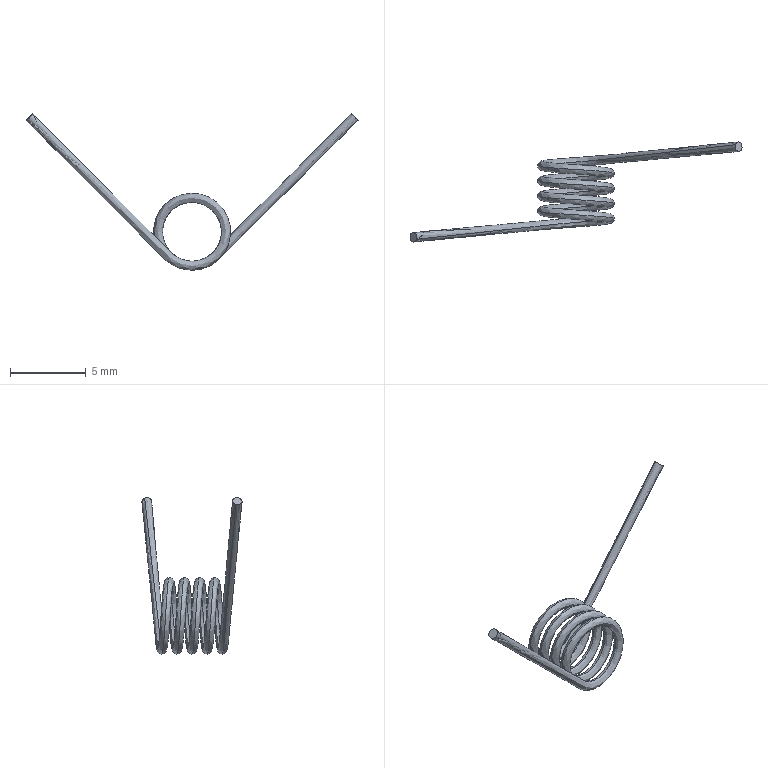Part | SolidWorks | features MoveFace 2, Helix 1, Sweep 1 | 1 solid | 4 faces | box 21.977 x 6.635 x 10.365 mm | volume 24.784 mm3 | spline 2 | plane 2